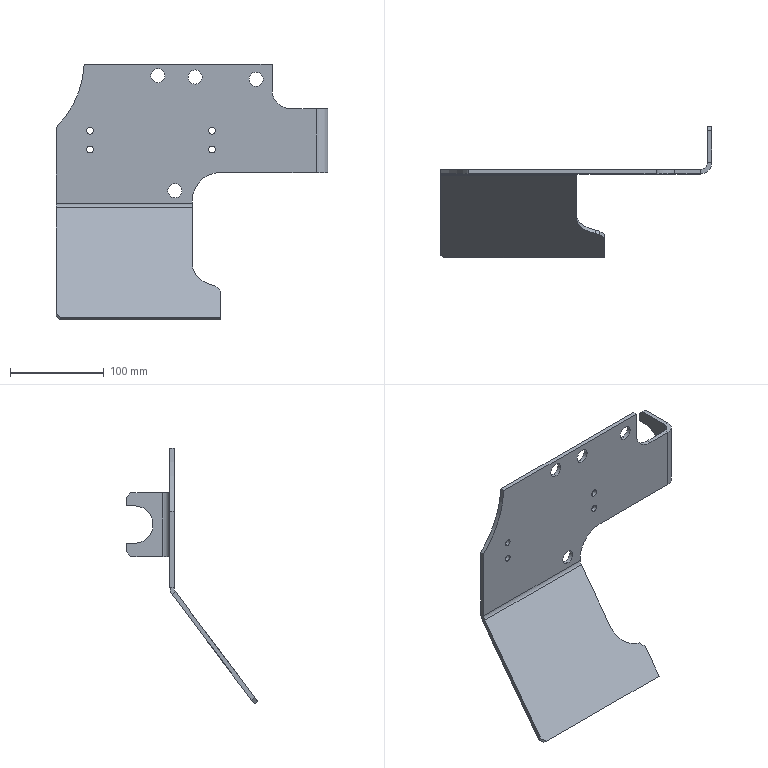Part | SolidWorks | features ICE 3, Chamfer 1, EdgeFlange 1, FlatPattern 1, SMBaseFlange 1, SheetMetal 1 | 1 solid | 56 faces | box 289.5 x 140.1 x 272.5 mm | volume 264608 mm3 | plane 31 | cylinder 25 | commonest cylinder face diameters 7.2 x8 15 x8 16 x2 25 x2 40 x2 60 x2